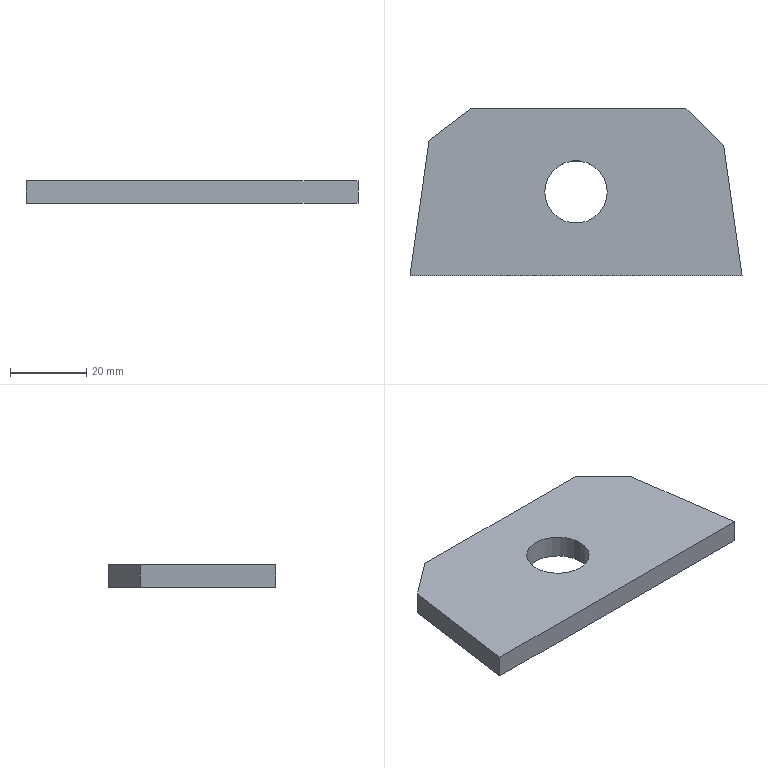Part | SolidWorks | features Chamfer 1, Extrusion 1, ICE 1 | 1 solid | 10 faces | box 87 x 44 x 6 mm | volume 19570 mm3 | plane 8 | cylinder 2 | commonest cylinder face diameters 16.358 x2
STEP:
#1=CARTESIAN_POINT('',(-8.179,0.,0.));
#2=VERTEX_POINT('',#1);
#3=CARTESIAN_POINT('',(8.179,0.,0.));
#4=VERTEX_POINT('',#3);
#5=CARTESIAN_POINT('',(0.,0.,0.));
#6=DIRECTION('',(0.,0.,1.));
#7=DIRECTION('',(1.,0.,0.));
#8=AXIS2_PLACEMENT_3D('',#5,#6,#7);
#9=CIRCLE('',#8,8.179);
#10=EDGE_CURVE('',#2,#4,#9,.T.);
#11=ORIENTED_EDGE('',*,*,#10,.F.);
#12=CARTESIAN_POINT('',(-8.179,0.,6.));
#13=VERTEX_POINT('',#12);
#14=CARTESIAN_POINT('',(-8.179,0.,0.));
#15=DIRECTION('',(0.,0.,1.));
#16=VECTOR('',#15,1000.);
#17=LINE('',#14,#16);
#18=EDGE_CURVE('',#2,#13,#17,.T.);
#19=ORIENTED_EDGE('',*,*,#18,.T.);
#20=CARTESIAN_POINT('',(8.179,0.,6.));
#21=VERTEX_POINT('',#20);
#22=CARTESIAN_POINT('',(0.,0.,6.));
#23=DIRECTION('',(0.,0.,1.));
#24=DIRECTION('',(1.,0.,0.));
#25=AXIS2_PLACEMENT_3D('',#22,#23,#24);
#26=CIRCLE('',#25,8.179);
#27=EDGE_CURVE('',#13,#21,#26,.T.);
#28=ORIENTED_EDGE('',*,*,#27,.T.);
#29=CARTESIAN_POINT('',(8.179,0.,0.));
#30=DIRECTION('',(0.,0.,1.));
#31=VECTOR('',#30,1000.);
#32=LINE('',#29,#31);
#33=EDGE_CURVE('',#4,#21,#32,.T.);
#34=ORIENTED_EDGE('',*,*,#33,.F.);
#35=EDGE_LOOP('',(#11,#19,#28,#34));
#36=FACE_OUTER_BOUND('',#35,.T.);
#37=CARTESIAN_POINT('',(0.,0.,0.));
#38=DIRECTION('',(0.,0.,1.));
#39=DIRECTION('',(1.,0.,0.));
#40=AXIS2_PLACEMENT_3D('',#37,#38,#39);
#41=CYLINDRICAL_SURFACE('',#40,8.179);
#42=ADVANCED_FACE('',(#36),#41,.F.);
#43=CARTESIAN_POINT('',(-43.5,-22.,0.));
#44=VERTEX_POINT('',#43);
#45=CARTESIAN_POINT('',(43.5,-22.,0.));
#46=VERTEX_POINT('',#45);
#47=CARTESIAN_POINT('',(43.5,-22.,0.));
#48=DIRECTION('',(1.,0.,0.));
#49=VECTOR('',#48,1000.);
#50=LINE('',#47,#49);
#51=EDGE_CURVE('',#44,#46,#50,.T.);
#52=ORIENTED_EDGE('',*,*,#51,.T.);
#53=CARTESIAN_POINT('',(43.5,-22.,6.));
#54=VERTEX_POINT('',#53);
#55=CARTESIAN_POINT('',(43.5,-22.,6.));
#56=DIRECTION('',(0.,0.,-1.));
#57=VECTOR('',#56,1000.);
#58=LINE('',#55,#57);
#59=EDGE_CURVE('',#54,#46,#58,.T.);
#60=ORIENTED_EDGE('',*,*,#59,.F.);
#61=CARTESIAN_POINT('',(-43.5,-22.,6.));
#62=VERTEX_POINT('',#61);
#63=CARTESIAN_POINT('',(43.5,-22.,6.));
#64=DIRECTION('',(1.,0.,0.));
#65=VECTOR('',#64,1000.);
#66=LINE('',#63,#65);
#67=EDGE_CURVE('',#62,#54,#66,.T.);
#68=ORIENTED_EDGE('',*,*,#67,.F.);
#69=CARTESIAN_POINT('',(-43.5,-22.,6.));
#70=DIRECTION('',(0.,0.,-1.));
#71=VECTOR('',#70,1000.);
#72=LINE('',#69,#71);
#73=EDGE_CURVE('',#62,#44,#72,.T.);
#74=ORIENTED_EDGE('',*,*,#73,.T.);
#75=EDGE_LOOP('',(#52,#60,#68,#74));
#76=FACE_OUTER_BOUND('',#75,.T.);
#77=CARTESIAN_POINT('',(43.5,-22.,6.));
#78=DIRECTION('',(0.,1.,0.));
#79=DIRECTION('',(-1.,0.,0.));
#80=AXIS2_PLACEMENT_3D('',#77,#78,#79);
#81=PLANE('',#80);
#82=ADVANCED_FACE('',(#76),#81,.F.);
#83=CARTESIAN_POINT('',(28.816,22.,6.));
#84=VERTEX_POINT('',#83);
#85=CARTESIAN_POINT('',(-27.329,22.,6.));
#86=VERTEX_POINT('',#85);
#87=CARTESIAN_POINT('',(43.5,22.,6.));
#88=DIRECTION('',(-1.,0.,0.));
#89=VECTOR('',#88,1000.);
#90=LINE('',#87,#89);
#91=EDGE_CURVE('',#84,#86,#90,.T.);
#92=ORIENTED_EDGE('',*,*,#91,.F.);
#93=CARTESIAN_POINT('',(28.816,22.,0.));
#94=VERTEX_POINT('',#93);
#95=CARTESIAN_POINT('',(28.816,22.,6.));
#96=DIRECTION('',(0.,0.,-1.));
#97=VECTOR('',#96,1000.);
#98=LINE('',#95,#97);
#99=EDGE_CURVE('',#84,#94,#98,.T.);
#100=ORIENTED_EDGE('',*,*,#99,.T.);
#101=CARTESIAN_POINT('',(-27.329,22.,0.));
#102=VERTEX_POINT('',#101);
#103=CARTESIAN_POINT('',(43.5,22.,0.));
#104=DIRECTION('',(-1.,0.,0.));
#105=VECTOR('',#104,1000.);
#106=LINE('',#103,#105);
#107=EDGE_CURVE('',#94,#102,#106,.T.);
#108=ORIENTED_EDGE('',*,*,#107,.T.);
#109=CARTESIAN_POINT('',(-27.329,22.,6.));
#110=DIRECTION('',(0.,0.,1.));
#111=VECTOR('',#110,1000.);
#112=LINE('',#109,#111);
#113=EDGE_CURVE('',#102,#86,#112,.T.);
#114=ORIENTED_EDGE('',*,*,#113,.T.);
#115=EDGE_LOOP('',(#92,#100,#108,#114));
#116=FACE_OUTER_BOUND('',#115,.T.);
#117=CARTESIAN_POINT('',(43.5,22.,6.));
#118=DIRECTION('',(0.,-1.,0.));
#119=DIRECTION('',(1.,0.,0.));
#120=AXIS2_PLACEMENT_3D('',#117,#118,#119);
#121=PLANE('',#120);
#122=ADVANCED_FACE('',(#116),#121,.F.);
#123=CARTESIAN_POINT('',(0.,0.,6.));
#124=DIRECTION('',(0.,0.,1.));
#125=DIRECTION('',(1.,0.,0.));
#126=AXIS2_PLACEMENT_3D('',#123,#124,#125);
#127=CIRCLE('',#126,8.179);
#128=EDGE_CURVE('',#21,#13,#127,.T.);
#129=ORIENTED_EDGE('',*,*,#128,.F.);
#130=ORIENTED_EDGE('',*,*,#27,.F.);
#131=EDGE_LOOP('',(#129,#130));
#132=FACE_BOUND('',#131,.T.);
#133=CARTESIAN_POINT('',(38.706,12.11,6.));
#134=VERTEX_POINT('',#133);
#135=CARTESIAN_POINT('',(43.5,-22.,6.));
#136=DIRECTION('',(0.1392,-0.9903,0.));
#137=VECTOR('',#136,1000.);
#138=LINE('',#135,#137);
#139=EDGE_CURVE('',#134,#54,#138,.T.);
#140=ORIENTED_EDGE('',*,*,#139,.F.);
#141=CARTESIAN_POINT('',(38.706,12.11,6.));
#142=DIRECTION('',(-0.7071,0.7071,0.));
#143=VECTOR('',#142,1000.);
#144=LINE('',#141,#143);
#145=EDGE_CURVE('',#134,#84,#144,.T.);
#146=ORIENTED_EDGE('',*,*,#145,.T.);
#147=ORIENTED_EDGE('',*,*,#91,.T.);
#148=CARTESIAN_POINT('',(-38.499,13.583,6.));
#149=VERTEX_POINT('',#148);
#150=CARTESIAN_POINT('',(-27.329,22.,6.));
#151=DIRECTION('',(-0.7986,-0.6018,0.));
#152=VECTOR('',#151,1000.);
#153=LINE('',#150,#152);
#154=EDGE_CURVE('',#86,#149,#153,.T.);
#155=ORIENTED_EDGE('',*,*,#154,.T.);
#156=CARTESIAN_POINT('',(-43.5,-22.,6.));
#157=DIRECTION('',(0.1392,0.9903,0.));
#158=VECTOR('',#157,1000.);
#159=LINE('',#156,#158);
#160=EDGE_CURVE('',#62,#149,#159,.T.);
#161=ORIENTED_EDGE('',*,*,#160,.F.);
#162=ORIENTED_EDGE('',*,*,#67,.T.);
#163=EDGE_LOOP('',(#140,#146,#147,#155,#161,#162));
#164=FACE_OUTER_BOUND('',#163,.T.);
#165=CARTESIAN_POINT('',(0.,0.,6.));
#166=DIRECTION('',(0.,0.,-1.));
#167=DIRECTION('',(-1.,0.,0.));
#168=AXIS2_PLACEMENT_3D('',#165,#166,#167);
#169=PLANE('',#168);
#170=ADVANCED_FACE('',(#132,#164),#169,.F.);
#171=ORIENTED_EDGE('',*,*,#107,.F.);
#172=CARTESIAN_POINT('',(38.706,12.11,0.));
#173=VERTEX_POINT('',#172);
#174=CARTESIAN_POINT('',(25.408,25.408,0.));
#175=DIRECTION('',(0.7071,-0.7071,0.));
#176=VECTOR('',#175,1000.);
#177=LINE('',#174,#176);
#178=EDGE_CURVE('',#94,#173,#177,.T.);
#179=ORIENTED_EDGE('',*,*,#178,.T.);
#180=CARTESIAN_POINT('',(43.5,-22.,0.));
#181=DIRECTION('',(0.1392,-0.9903,0.));
#182=VECTOR('',#181,1000.);
#183=LINE('',#180,#182);
#184=EDGE_CURVE('',#173,#46,#183,.T.);
#185=ORIENTED_EDGE('',*,*,#184,.T.);
#186=ORIENTED_EDGE('',*,*,#51,.F.);
#187=CARTESIAN_POINT('',(-38.499,13.583,0.));
#188=VERTEX_POINT('',#187);
#189=CARTESIAN_POINT('',(-43.5,-22.,0.));
#190=DIRECTION('',(0.1392,0.9903,0.));
#191=VECTOR('',#190,1000.);
#192=LINE('',#189,#191);
#193=EDGE_CURVE('',#44,#188,#192,.T.);
#194=ORIENTED_EDGE('',*,*,#193,.T.);
#195=CARTESIAN_POINT('',(-20.472,27.167,0.));
#196=DIRECTION('',(0.7986,0.6018,0.));
#197=VECTOR('',#196,1000.);
#198=LINE('',#195,#197);
#199=EDGE_CURVE('',#188,#102,#198,.T.);
#200=ORIENTED_EDGE('',*,*,#199,.T.);
#201=EDGE_LOOP('',(#171,#179,#185,#186,#194,#200));
#202=FACE_OUTER_BOUND('',#201,.T.);
#203=CARTESIAN_POINT('',(0.,0.,0.));
#204=DIRECTION('',(0.,0.,1.));
#205=DIRECTION('',(1.,0.,0.));
#206=AXIS2_PLACEMENT_3D('',#203,#204,#205);
#207=CIRCLE('',#206,8.179);
#208=EDGE_CURVE('',#4,#2,#207,.T.);
#209=ORIENTED_EDGE('',*,*,#208,.T.);
#210=ORIENTED_EDGE('',*,*,#10,.T.);
#211=EDGE_LOOP('',(#209,#210));
#212=FACE_BOUND('',#211,.T.);
#213=CARTESIAN_POINT('',(0.,0.,0.));
#214=DIRECTION('',(0.,0.,-1.));
#215=DIRECTION('',(-1.,0.,0.));
#216=AXIS2_PLACEMENT_3D('',#213,#214,#215);
#217=PLANE('',#216);
#218=ADVANCED_FACE('',(#202,#212),#217,.T.);
#219=ORIENTED_EDGE('',*,*,#18,.F.);
#220=ORIENTED_EDGE('',*,*,#208,.F.);
#221=ORIENTED_EDGE('',*,*,#33,.T.);
#222=ORIENTED_EDGE('',*,*,#128,.T.);
#223=EDGE_LOOP('',(#219,#220,#221,#222));
#224=FACE_OUTER_BOUND('',#223,.T.);
#225=CARTESIAN_POINT('',(0.,0.,0.));
#226=DIRECTION('',(0.,0.,1.));
#227=DIRECTION('',(1.,0.,0.));
#228=AXIS2_PLACEMENT_3D('',#225,#226,#227);
#229=CYLINDRICAL_SURFACE('',#228,8.179);
#230=ADVANCED_FACE('',(#224),#229,.F.);
#231=ORIENTED_EDGE('',*,*,#160,.T.);
#232=CARTESIAN_POINT('',(-38.499,13.583,0.));
#233=DIRECTION('',(0.,0.,-1.));
#234=VECTOR('',#233,1000.);
#235=LINE('',#232,#234);
#236=EDGE_CURVE('',#149,#188,#235,.T.);
#237=ORIENTED_EDGE('',*,*,#236,.T.);
#238=ORIENTED_EDGE('',*,*,#193,.F.);
#239=ORIENTED_EDGE('',*,*,#73,.F.);
#240=EDGE_LOOP('',(#231,#237,#238,#239));
#241=FACE_OUTER_BOUND('',#240,.T.);
#242=CARTESIAN_POINT('',(-43.5,-22.,0.));
#243=DIRECTION('',(0.9903,-0.1392,0.));
#244=DIRECTION('',(0.1392,0.9903,0.));
#245=AXIS2_PLACEMENT_3D('',#242,#243,#244);
#246=PLANE('',#245);
#247=ADVANCED_FACE('',(#241),#246,.F.);
#248=ORIENTED_EDGE('',*,*,#184,.F.);
#249=CARTESIAN_POINT('',(38.706,12.11,0.));
#250=DIRECTION('',(0.,0.,1.));
#251=VECTOR('',#250,1000.);
#252=LINE('',#249,#251);
#253=EDGE_CURVE('',#173,#134,#252,.T.);
#254=ORIENTED_EDGE('',*,*,#253,.T.);
#255=ORIENTED_EDGE('',*,*,#139,.T.);
#256=ORIENTED_EDGE('',*,*,#59,.T.);
#257=EDGE_LOOP('',(#248,#254,#255,#256));
#258=FACE_OUTER_BOUND('',#257,.T.);
#259=CARTESIAN_POINT('',(43.5,-22.,0.));
#260=DIRECTION('',(-0.9903,-0.1392,0.));
#261=DIRECTION('',(0.1392,-0.9903,0.));
#262=AXIS2_PLACEMENT_3D('',#259,#260,#261);
#263=PLANE('',#262);
#264=ADVANCED_FACE('',(#258),#263,.F.);
#265=ORIENTED_EDGE('',*,*,#178,.F.);
#266=ORIENTED_EDGE('',*,*,#99,.F.);
#267=ORIENTED_EDGE('',*,*,#145,.F.);
#268=ORIENTED_EDGE('',*,*,#253,.F.);
#269=EDGE_LOOP('',(#265,#266,#267,#268));
#270=FACE_OUTER_BOUND('',#269,.T.);
#271=CARTESIAN_POINT('',(38.706,12.11,0.));
#272=DIRECTION('',(-0.7071,-0.7071,0.));
#273=DIRECTION('',(0.,0.,1.));
#274=AXIS2_PLACEMENT_3D('',#271,#272,#273);
#275=PLANE('',#274);
#276=ADVANCED_FACE('',(#270),#275,.F.);
#277=ORIENTED_EDGE('',*,*,#199,.F.);
#278=ORIENTED_EDGE('',*,*,#236,.F.);
#279=ORIENTED_EDGE('',*,*,#154,.F.);
#280=ORIENTED_EDGE('',*,*,#113,.F.);
#281=EDGE_LOOP('',(#277,#278,#279,#280));
#282=FACE_OUTER_BOUND('',#281,.T.);
#283=CARTESIAN_POINT('',(-27.329,22.,6.));
#284=DIRECTION('',(0.6018,-0.7986,0.));
#285=DIRECTION('',(0.,0.,1.));
#286=AXIS2_PLACEMENT_3D('',#283,#284,#285);
#287=PLANE('',#286);
#288=ADVANCED_FACE('',(#282),#287,.F.);
#289=CLOSED_SHELL('',(#42,#82,#122,#170,#218,#230,#247,#264,#276,#288));
#290=MANIFOLD_SOLID_BREP('',#289);
#291=CARTESIAN_POINT('',(0.,0.,0.));
#292=DIRECTION('',(0.,0.,1.));
#293=DIRECTION('',(1.,0.,0.));
#294=AXIS2_PLACEMENT_3D('',#291,#292,#293);
#295=(LENGTH_UNIT()NAMED_UNIT(*)SI_UNIT(.MILLI.,.METRE.));
#296=UNCERTAINTY_MEASURE_WITH_UNIT(LENGTH_MEASURE(0.00001),#295,'','');
#297=(NAMED_UNIT(*)PLANE_ANGLE_UNIT()SI_UNIT($,.RADIAN.));
#298=(NAMED_UNIT(*)SI_UNIT($,.STERADIAN.)SOLID_ANGLE_UNIT());
#299=(GEOMETRIC_REPRESENTATION_CONTEXT(3)GLOBAL_UNCERTAINTY_ASSIGNED_CONTEXT((#296))GLOBAL_UNIT_ASSIGNED_CONTEXT((#295,#297,#298))REPRESENTATION_CONTEXT('',''));
#300=ADVANCED_BREP_SHAPE_REPRESENTATION('',(#290,#294),#299);